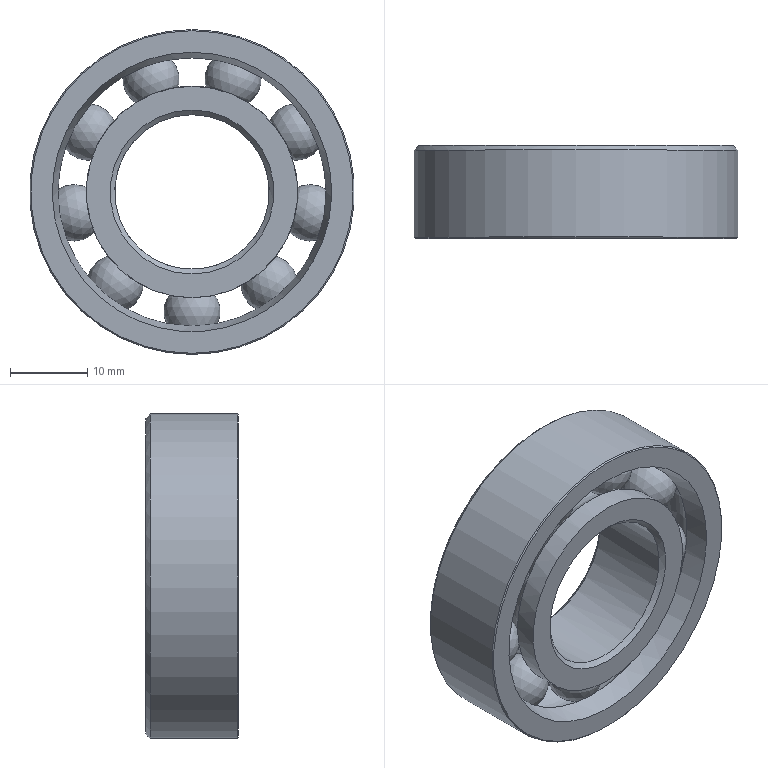Part | STEP file | YBQDJ-YB-29 | 1 solid | 41 faces | box 42 x 12 x 42 mm | volume 8686 mm3 | torus 18 | sphere 9 | cylinder 5 | cone 5 | plane 4 | commonest cylinder face diameters 27.334 x2 20 x1 34.666 x1 42 x1